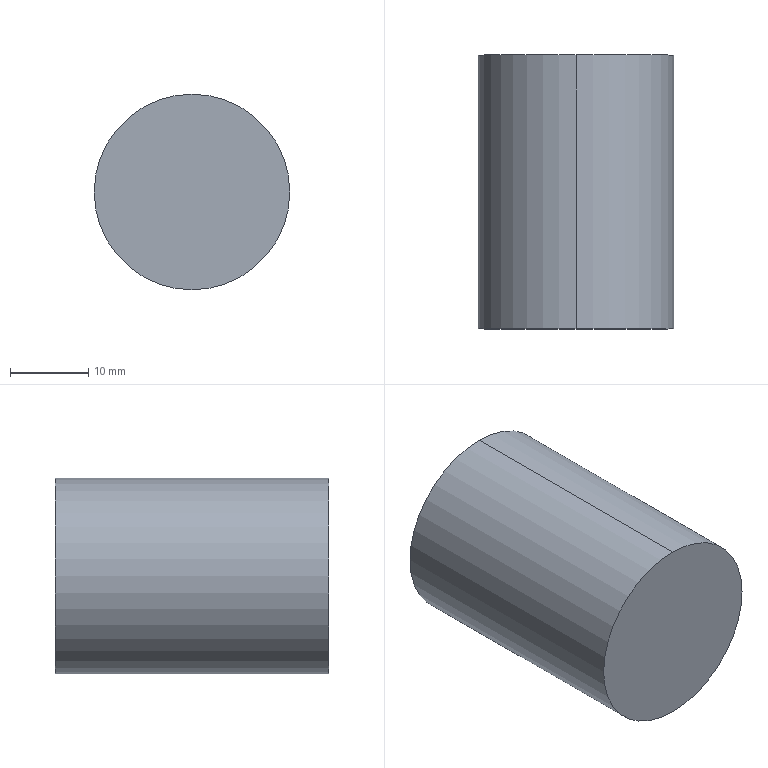Part | SolidWorks | features Revolution 1 | 1 solid | 4 faces | box 25 x 35 x 25 mm | volume 17181 mm3 | cylinder 2 | plane 2 | commonest cylinder face diameters 25 x2
STEP:
#1=CARTESIAN_POINT('',(0.,35.,-12.5));
#2=VERTEX_POINT('',#1);
#3=CARTESIAN_POINT('',(0.,35.,12.5));
#4=VERTEX_POINT('',#3);
#5=CARTESIAN_POINT('',(0.,35.,0.));
#6=DIRECTION('',(0.,-1.,0.));
#7=DIRECTION('',(0.,0.,-1.));
#8=AXIS2_PLACEMENT_3D('',#5,#6,#7);
#9=CIRCLE('',#8,12.5);
#10=EDGE_CURVE('',#2,#4,#9,.T.);
#11=ORIENTED_EDGE('',*,*,#10,.T.);
#12=CARTESIAN_POINT('',(0.,0.,12.5));
#13=VERTEX_POINT('',#12);
#14=CARTESIAN_POINT('',(0.,0.,12.5));
#15=DIRECTION('',(0.,-1.,0.));
#16=VECTOR('',#15,1000.);
#17=LINE('',#14,#16);
#18=EDGE_CURVE('',#4,#13,#17,.T.);
#19=ORIENTED_EDGE('',*,*,#18,.T.);
#20=CARTESIAN_POINT('',(0.,0.,-12.5));
#21=VERTEX_POINT('',#20);
#22=CARTESIAN_POINT('',(0.,0.,0.));
#23=DIRECTION('',(0.,-1.,0.));
#24=DIRECTION('',(0.,0.,-1.));
#25=AXIS2_PLACEMENT_3D('',#22,#23,#24);
#26=CIRCLE('',#25,12.5);
#27=EDGE_CURVE('',#21,#13,#26,.T.);
#28=ORIENTED_EDGE('',*,*,#27,.F.);
#29=CARTESIAN_POINT('',(0.,0.,-12.5));
#30=DIRECTION('',(0.,-1.,0.));
#31=VECTOR('',#30,1000.);
#32=LINE('',#29,#31);
#33=EDGE_CURVE('',#2,#21,#32,.T.);
#34=ORIENTED_EDGE('',*,*,#33,.F.);
#35=EDGE_LOOP('',(#11,#19,#28,#34));
#36=FACE_OUTER_BOUND('',#35,.T.);
#37=CARTESIAN_POINT('',(0.,0.,0.));
#38=DIRECTION('',(0.,-1.,0.));
#39=DIRECTION('',(0.,0.,-1.));
#40=AXIS2_PLACEMENT_3D('',#37,#38,#39);
#41=CYLINDRICAL_SURFACE('',#40,12.5);
#42=ADVANCED_FACE('',(#36),#41,.T.);
#43=ORIENTED_EDGE('',*,*,#10,.F.);
#44=CARTESIAN_POINT('',(0.,35.,0.));
#45=DIRECTION('',(0.,-1.,0.));
#46=DIRECTION('',(0.,0.,-1.));
#47=AXIS2_PLACEMENT_3D('',#44,#45,#46);
#48=CIRCLE('',#47,12.5);
#49=EDGE_CURVE('',#4,#2,#48,.T.);
#50=ORIENTED_EDGE('',*,*,#49,.F.);
#51=EDGE_LOOP('',(#43,#50));
#52=FACE_OUTER_BOUND('',#51,.T.);
#53=CARTESIAN_POINT('',(0.,35.,0.));
#54=DIRECTION('',(0.,-1.,0.));
#55=DIRECTION('',(0.,0.,-1.));
#56=AXIS2_PLACEMENT_3D('',#53,#54,#55);
#57=PLANE('',#56);
#58=ADVANCED_FACE('',(#52),#57,.F.);
#59=ORIENTED_EDGE('',*,*,#18,.F.);
#60=ORIENTED_EDGE('',*,*,#49,.T.);
#61=ORIENTED_EDGE('',*,*,#33,.T.);
#62=CARTESIAN_POINT('',(0.,0.,0.));
#63=DIRECTION('',(0.,-1.,0.));
#64=DIRECTION('',(0.,0.,-1.));
#65=AXIS2_PLACEMENT_3D('',#62,#63,#64);
#66=CIRCLE('',#65,12.5);
#67=EDGE_CURVE('',#13,#21,#66,.T.);
#68=ORIENTED_EDGE('',*,*,#67,.F.);
#69=EDGE_LOOP('',(#59,#60,#61,#68));
#70=FACE_OUTER_BOUND('',#69,.T.);
#71=CARTESIAN_POINT('',(0.,0.,0.));
#72=DIRECTION('',(0.,-1.,0.));
#73=DIRECTION('',(0.,0.,-1.));
#74=AXIS2_PLACEMENT_3D('',#71,#72,#73);
#75=CYLINDRICAL_SURFACE('',#74,12.5);
#76=ADVANCED_FACE('',(#70),#75,.T.);
#77=ORIENTED_EDGE('',*,*,#27,.T.);
#78=ORIENTED_EDGE('',*,*,#67,.T.);
#79=EDGE_LOOP('',(#77,#78));
#80=FACE_OUTER_BOUND('',#79,.T.);
#81=CARTESIAN_POINT('',(0.,0.,0.));
#82=DIRECTION('',(0.,1.,0.));
#83=DIRECTION('',(0.,0.,1.));
#84=AXIS2_PLACEMENT_3D('',#81,#82,#83);
#85=PLANE('',#84);
#86=ADVANCED_FACE('',(#80),#85,.F.);
#87=CLOSED_SHELL('',(#42,#58,#76,#86));
#88=MANIFOLD_SOLID_BREP('',#87);
#89=CARTESIAN_POINT('',(0.,0.,0.));
#90=DIRECTION('',(0.,0.,1.));
#91=DIRECTION('',(1.,0.,0.));
#92=AXIS2_PLACEMENT_3D('',#89,#90,#91);
#93=(LENGTH_UNIT()NAMED_UNIT(*)SI_UNIT(.MILLI.,.METRE.));
#94=UNCERTAINTY_MEASURE_WITH_UNIT(LENGTH_MEASURE(0.00001),#93,'','');
#95=(NAMED_UNIT(*)PLANE_ANGLE_UNIT()SI_UNIT($,.RADIAN.));
#96=(NAMED_UNIT(*)SI_UNIT($,.STERADIAN.)SOLID_ANGLE_UNIT());
#97=(GEOMETRIC_REPRESENTATION_CONTEXT(3)GLOBAL_UNCERTAINTY_ASSIGNED_CONTEXT((#94))GLOBAL_UNIT_ASSIGNED_CONTEXT((#93,#95,#96))REPRESENTATION_CONTEXT('',''));
#98=ADVANCED_BREP_SHAPE_REPRESENTATION('',(#88,#92),#97);